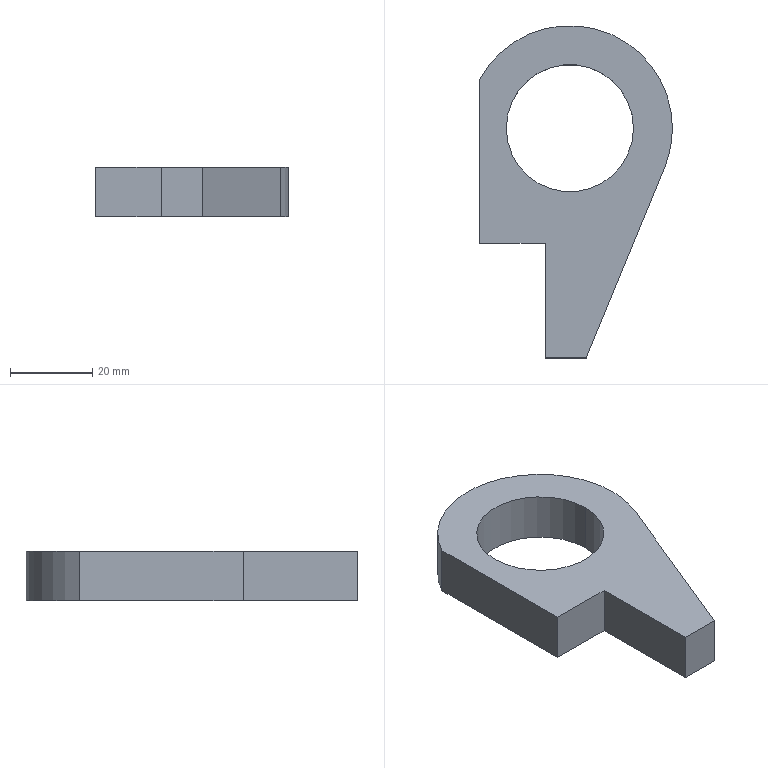Part | SolidWorks | features FlatPattern 1, SMBaseFlange 1, SheetMetal 1 | 1 solid | 11 faces | box 47 x 81 x 12 mm | volume 22191 mm3 | plane 7 | cylinder 4 | commonest cylinder face diameters 31 x2 50 x2
STEP:
#1=CARTESIAN_POINT('',(-15.5,0.,-12.));
#2=VERTEX_POINT('',#1);
#3=CARTESIAN_POINT('',(15.5,0.,-12.));
#4=VERTEX_POINT('',#3);
#5=CARTESIAN_POINT('',(0.,0.,-12.));
#6=DIRECTION('',(0.,0.,1.));
#7=DIRECTION('',(1.,0.,0.));
#8=AXIS2_PLACEMENT_3D('',#5,#6,#7);
#9=CIRCLE('',#8,15.5);
#10=EDGE_CURVE('',#2,#4,#9,.T.);
#11=ORIENTED_EDGE('',*,*,#10,.F.);
#12=CARTESIAN_POINT('',(-15.5,0.,0.));
#13=VERTEX_POINT('',#12);
#14=CARTESIAN_POINT('',(-15.5,0.,-12.));
#15=DIRECTION('',(0.,0.,1.));
#16=VECTOR('',#15,1000.);
#17=LINE('',#14,#16);
#18=EDGE_CURVE('',#2,#13,#17,.T.);
#19=ORIENTED_EDGE('',*,*,#18,.T.);
#20=CARTESIAN_POINT('',(15.5,0.,0.));
#21=VERTEX_POINT('',#20);
#22=CARTESIAN_POINT('',(0.,0.,0.));
#23=DIRECTION('',(0.,0.,1.));
#24=DIRECTION('',(1.,0.,0.));
#25=AXIS2_PLACEMENT_3D('',#22,#23,#24);
#26=CIRCLE('',#25,15.5);
#27=EDGE_CURVE('',#13,#21,#26,.T.);
#28=ORIENTED_EDGE('',*,*,#27,.T.);
#29=CARTESIAN_POINT('',(15.5,0.,-12.));
#30=DIRECTION('',(0.,0.,1.));
#31=VECTOR('',#30,1000.);
#32=LINE('',#29,#31);
#33=EDGE_CURVE('',#4,#21,#32,.T.);
#34=ORIENTED_EDGE('',*,*,#33,.F.);
#35=EDGE_LOOP('',(#11,#19,#28,#34));
#36=FACE_OUTER_BOUND('',#35,.T.);
#37=CARTESIAN_POINT('',(0.,0.,-12.));
#38=DIRECTION('',(0.,0.,1.));
#39=DIRECTION('',(1.,0.,0.));
#40=AXIS2_PLACEMENT_3D('',#37,#38,#39);
#41=CYLINDRICAL_SURFACE('',#40,15.5);
#42=ADVANCED_FACE('',(#36),#41,.F.);
#43=CARTESIAN_POINT('',(23.121,-9.509,-12.));
#44=VERTEX_POINT('',#43);
#45=CARTESIAN_POINT('',(25.,0.,-12.));
#46=VERTEX_POINT('',#45);
#47=CARTESIAN_POINT('',(0.,0.,-12.));
#48=DIRECTION('',(0.,0.,1.));
#49=DIRECTION('',(1.,0.,0.));
#50=AXIS2_PLACEMENT_3D('',#47,#48,#49);
#51=CIRCLE('',#50,25.);
#52=EDGE_CURVE('',#44,#46,#51,.T.);
#53=ORIENTED_EDGE('',*,*,#52,.T.);
#54=CARTESIAN_POINT('',(25.,0.,0.));
#55=VERTEX_POINT('',#54);
#56=CARTESIAN_POINT('',(25.,0.,-12.));
#57=DIRECTION('',(0.,0.,1.));
#58=VECTOR('',#57,1000.);
#59=LINE('',#56,#58);
#60=EDGE_CURVE('',#46,#55,#59,.T.);
#61=ORIENTED_EDGE('',*,*,#60,.T.);
#62=CARTESIAN_POINT('',(23.121,-9.509,0.));
#63=VERTEX_POINT('',#62);
#64=CARTESIAN_POINT('',(0.,0.,0.));
#65=DIRECTION('',(0.,0.,1.));
#66=DIRECTION('',(1.,0.,0.));
#67=AXIS2_PLACEMENT_3D('',#64,#65,#66);
#68=CIRCLE('',#67,25.);
#69=EDGE_CURVE('',#63,#55,#68,.T.);
#70=ORIENTED_EDGE('',*,*,#69,.F.);
#71=CARTESIAN_POINT('',(23.121,-9.509,-12.));
#72=DIRECTION('',(0.,0.,1.));
#73=VECTOR('',#72,1000.);
#74=LINE('',#71,#73);
#75=EDGE_CURVE('',#44,#63,#74,.T.);
#76=ORIENTED_EDGE('',*,*,#75,.F.);
#77=EDGE_LOOP('',(#53,#61,#70,#76));
#78=FACE_OUTER_BOUND('',#77,.T.);
#79=CARTESIAN_POINT('',(0.,0.,-12.));
#80=DIRECTION('',(0.,0.,1.));
#81=DIRECTION('',(1.,0.,0.));
#82=AXIS2_PLACEMENT_3D('',#79,#80,#81);
#83=CYLINDRICAL_SURFACE('',#82,25.);
#84=ADVANCED_FACE('',(#78),#83,.T.);
#85=ORIENTED_EDGE('',*,*,#60,.F.);
#86=CARTESIAN_POINT('',(-22.,11.874,-12.));
#87=VERTEX_POINT('',#86);
#88=CARTESIAN_POINT('',(0.,0.,-12.));
#89=DIRECTION('',(0.,0.,1.));
#90=DIRECTION('',(1.,0.,0.));
#91=AXIS2_PLACEMENT_3D('',#88,#89,#90);
#92=CIRCLE('',#91,25.);
#93=EDGE_CURVE('',#46,#87,#92,.T.);
#94=ORIENTED_EDGE('',*,*,#93,.T.);
#95=CARTESIAN_POINT('',(-22.,11.874,0.));
#96=VERTEX_POINT('',#95);
#97=CARTESIAN_POINT('',(-22.,11.874,-12.));
#98=DIRECTION('',(0.,0.,1.));
#99=VECTOR('',#98,1000.);
#100=LINE('',#97,#99);
#101=EDGE_CURVE('',#87,#96,#100,.T.);
#102=ORIENTED_EDGE('',*,*,#101,.T.);
#103=CARTESIAN_POINT('',(0.,0.,0.));
#104=DIRECTION('',(0.,0.,1.));
#105=DIRECTION('',(1.,0.,0.));
#106=AXIS2_PLACEMENT_3D('',#103,#104,#105);
#107=CIRCLE('',#106,25.);
#108=EDGE_CURVE('',#55,#96,#107,.T.);
#109=ORIENTED_EDGE('',*,*,#108,.F.);
#110=EDGE_LOOP('',(#85,#94,#102,#109));
#111=FACE_OUTER_BOUND('',#110,.T.);
#112=CARTESIAN_POINT('',(0.,0.,-12.));
#113=DIRECTION('',(0.,0.,1.));
#114=DIRECTION('',(1.,0.,0.));
#115=AXIS2_PLACEMENT_3D('',#112,#113,#114);
#116=CYLINDRICAL_SURFACE('',#115,25.);
#117=ADVANCED_FACE('',(#111),#116,.T.);
#118=CARTESIAN_POINT('',(4.,-56.,0.));
#119=VERTEX_POINT('',#118);
#120=CARTESIAN_POINT('',(4.,-56.,0.));
#121=DIRECTION('',(0.3804,0.9248,0.));
#122=VECTOR('',#121,1000.);
#123=LINE('',#120,#122);
#124=EDGE_CURVE('',#119,#63,#123,.T.);
#125=ORIENTED_EDGE('',*,*,#124,.F.);
#126=CARTESIAN_POINT('',(4.,-56.,-12.));
#127=VERTEX_POINT('',#126);
#128=CARTESIAN_POINT('',(4.,-56.,-12.));
#129=DIRECTION('',(0.,0.,1.));
#130=VECTOR('',#129,1000.);
#131=LINE('',#128,#130);
#132=EDGE_CURVE('',#127,#119,#131,.T.);
#133=ORIENTED_EDGE('',*,*,#132,.F.);
#134=CARTESIAN_POINT('',(4.,-56.,-12.));
#135=DIRECTION('',(0.3804,0.9248,0.));
#136=VECTOR('',#135,1000.);
#137=LINE('',#134,#136);
#138=EDGE_CURVE('',#127,#44,#137,.T.);
#139=ORIENTED_EDGE('',*,*,#138,.T.);
#140=ORIENTED_EDGE('',*,*,#75,.T.);
#141=EDGE_LOOP('',(#125,#133,#139,#140));
#142=FACE_OUTER_BOUND('',#141,.T.);
#143=CARTESIAN_POINT('',(4.,-56.,-12.));
#144=DIRECTION('',(0.9248,-0.3804,0.));
#145=DIRECTION('',(0.3804,0.9248,0.));
#146=AXIS2_PLACEMENT_3D('',#143,#144,#145);
#147=PLANE('',#146);
#148=ADVANCED_FACE('',(#142),#147,.T.);
#149=CARTESIAN_POINT('',(-6.,-56.,0.));
#150=VERTEX_POINT('',#149);
#151=CARTESIAN_POINT('',(-6.,-56.,0.));
#152=DIRECTION('',(1.,0.,0.));
#153=VECTOR('',#152,1000.);
#154=LINE('',#151,#153);
#155=EDGE_CURVE('',#150,#119,#154,.T.);
#156=ORIENTED_EDGE('',*,*,#155,.F.);
#157=CARTESIAN_POINT('',(-6.,-56.,-12.));
#158=VERTEX_POINT('',#157);
#159=CARTESIAN_POINT('',(-6.,-56.,-12.));
#160=DIRECTION('',(0.,0.,1.));
#161=VECTOR('',#160,1000.);
#162=LINE('',#159,#161);
#163=EDGE_CURVE('',#158,#150,#162,.T.);
#164=ORIENTED_EDGE('',*,*,#163,.F.);
#165=CARTESIAN_POINT('',(-6.,-56.,-12.));
#166=DIRECTION('',(1.,0.,0.));
#167=VECTOR('',#166,1000.);
#168=LINE('',#165,#167);
#169=EDGE_CURVE('',#158,#127,#168,.T.);
#170=ORIENTED_EDGE('',*,*,#169,.T.);
#171=ORIENTED_EDGE('',*,*,#132,.T.);
#172=EDGE_LOOP('',(#156,#164,#170,#171));
#173=FACE_OUTER_BOUND('',#172,.T.);
#174=CARTESIAN_POINT('',(-6.,-56.,-12.));
#175=DIRECTION('',(0.,-1.,0.));
#176=DIRECTION('',(0.,0.,-1.));
#177=AXIS2_PLACEMENT_3D('',#174,#175,#176);
#178=PLANE('',#177);
#179=ADVANCED_FACE('',(#173),#178,.T.);
#180=CARTESIAN_POINT('',(-6.,-28.,0.));
#181=VERTEX_POINT('',#180);
#182=CARTESIAN_POINT('',(-6.,-28.,0.));
#183=DIRECTION('',(0.,-1.,0.));
#184=VECTOR('',#183,1000.);
#185=LINE('',#182,#184);
#186=EDGE_CURVE('',#181,#150,#185,.T.);
#187=ORIENTED_EDGE('',*,*,#186,.F.);
#188=CARTESIAN_POINT('',(-6.,-28.,-12.));
#189=VERTEX_POINT('',#188);
#190=CARTESIAN_POINT('',(-6.,-28.,-12.));
#191=DIRECTION('',(0.,0.,1.));
#192=VECTOR('',#191,1000.);
#193=LINE('',#190,#192);
#194=EDGE_CURVE('',#189,#181,#193,.T.);
#195=ORIENTED_EDGE('',*,*,#194,.F.);
#196=CARTESIAN_POINT('',(-6.,-28.,-12.));
#197=DIRECTION('',(0.,-1.,0.));
#198=VECTOR('',#197,1000.);
#199=LINE('',#196,#198);
#200=EDGE_CURVE('',#189,#158,#199,.T.);
#201=ORIENTED_EDGE('',*,*,#200,.T.);
#202=ORIENTED_EDGE('',*,*,#163,.T.);
#203=EDGE_LOOP('',(#187,#195,#201,#202));
#204=FACE_OUTER_BOUND('',#203,.T.);
#205=CARTESIAN_POINT('',(-6.,-28.,-12.));
#206=DIRECTION('',(-1.,0.,0.));
#207=DIRECTION('',(0.,-1.,0.));
#208=AXIS2_PLACEMENT_3D('',#205,#206,#207);
#209=PLANE('',#208);
#210=ADVANCED_FACE('',(#204),#209,.T.);
#211=CARTESIAN_POINT('',(-22.,-28.,0.));
#212=VERTEX_POINT('',#211);
#213=CARTESIAN_POINT('',(-22.,-28.,0.));
#214=DIRECTION('',(1.,0.,0.));
#215=VECTOR('',#214,1000.);
#216=LINE('',#213,#215);
#217=EDGE_CURVE('',#212,#181,#216,.T.);
#218=ORIENTED_EDGE('',*,*,#217,.F.);
#219=CARTESIAN_POINT('',(-22.,-28.,-12.));
#220=VERTEX_POINT('',#219);
#221=CARTESIAN_POINT('',(-22.,-28.,-12.));
#222=DIRECTION('',(0.,0.,1.));
#223=VECTOR('',#222,1000.);
#224=LINE('',#221,#223);
#225=EDGE_CURVE('',#220,#212,#224,.T.);
#226=ORIENTED_EDGE('',*,*,#225,.F.);
#227=CARTESIAN_POINT('',(-22.,-28.,-12.));
#228=DIRECTION('',(1.,0.,0.));
#229=VECTOR('',#228,1000.);
#230=LINE('',#227,#229);
#231=EDGE_CURVE('',#220,#189,#230,.T.);
#232=ORIENTED_EDGE('',*,*,#231,.T.);
#233=ORIENTED_EDGE('',*,*,#194,.T.);
#234=EDGE_LOOP('',(#218,#226,#232,#233));
#235=FACE_OUTER_BOUND('',#234,.T.);
#236=CARTESIAN_POINT('',(-22.,-28.,-12.));
#237=DIRECTION('',(0.,-1.,0.));
#238=DIRECTION('',(0.,0.,-1.));
#239=AXIS2_PLACEMENT_3D('',#236,#237,#238);
#240=PLANE('',#239);
#241=ADVANCED_FACE('',(#235),#240,.T.);
#242=CARTESIAN_POINT('',(-22.,-28.,0.));
#243=DIRECTION('',(0.,-1.,0.));
#244=VECTOR('',#243,1000.);
#245=LINE('',#242,#244);
#246=EDGE_CURVE('',#96,#212,#245,.T.);
#247=ORIENTED_EDGE('',*,*,#246,.F.);
#248=ORIENTED_EDGE('',*,*,#101,.F.);
#249=CARTESIAN_POINT('',(-22.,-28.,-12.));
#250=DIRECTION('',(0.,-1.,0.));
#251=VECTOR('',#250,1000.);
#252=LINE('',#249,#251);
#253=EDGE_CURVE('',#87,#220,#252,.T.);
#254=ORIENTED_EDGE('',*,*,#253,.T.);
#255=ORIENTED_EDGE('',*,*,#225,.T.);
#256=EDGE_LOOP('',(#247,#248,#254,#255));
#257=FACE_OUTER_BOUND('',#256,.T.);
#258=CARTESIAN_POINT('',(-22.,-28.,-12.));
#259=DIRECTION('',(-1.,0.,0.));
#260=DIRECTION('',(0.,0.,1.));
#261=AXIS2_PLACEMENT_3D('',#258,#259,#260);
#262=PLANE('',#261);
#263=ADVANCED_FACE('',(#257),#262,.T.);
#264=CARTESIAN_POINT('',(0.,0.,-12.));
#265=DIRECTION('',(0.,0.,1.));
#266=DIRECTION('',(1.,0.,0.));
#267=AXIS2_PLACEMENT_3D('',#264,#265,#266);
#268=CIRCLE('',#267,15.5);
#269=EDGE_CURVE('',#4,#2,#268,.T.);
#270=ORIENTED_EDGE('',*,*,#269,.T.);
#271=ORIENTED_EDGE('',*,*,#10,.T.);
#272=EDGE_LOOP('',(#270,#271));
#273=FACE_BOUND('',#272,.T.);
#274=ORIENTED_EDGE('',*,*,#52,.F.);
#275=ORIENTED_EDGE('',*,*,#138,.F.);
#276=ORIENTED_EDGE('',*,*,#169,.F.);
#277=ORIENTED_EDGE('',*,*,#200,.F.);
#278=ORIENTED_EDGE('',*,*,#231,.F.);
#279=ORIENTED_EDGE('',*,*,#253,.F.);
#280=ORIENTED_EDGE('',*,*,#93,.F.);
#281=EDGE_LOOP('',(#274,#275,#276,#277,#278,#279,#280));
#282=FACE_OUTER_BOUND('',#281,.T.);
#283=CARTESIAN_POINT('',(0.,0.,-12.));
#284=DIRECTION('',(0.,0.,1.));
#285=DIRECTION('',(1.,0.,0.));
#286=AXIS2_PLACEMENT_3D('',#283,#284,#285);
#287=PLANE('',#286);
#288=ADVANCED_FACE('',(#273,#282),#287,.F.);
#289=CARTESIAN_POINT('',(0.,0.,0.));
#290=DIRECTION('',(0.,0.,1.));
#291=DIRECTION('',(1.,0.,0.));
#292=AXIS2_PLACEMENT_3D('',#289,#290,#291);
#293=CIRCLE('',#292,15.5);
#294=EDGE_CURVE('',#21,#13,#293,.T.);
#295=ORIENTED_EDGE('',*,*,#294,.F.);
#296=ORIENTED_EDGE('',*,*,#27,.F.);
#297=EDGE_LOOP('',(#295,#296));
#298=FACE_BOUND('',#297,.T.);
#299=ORIENTED_EDGE('',*,*,#69,.T.);
#300=ORIENTED_EDGE('',*,*,#108,.T.);
#301=ORIENTED_EDGE('',*,*,#246,.T.);
#302=ORIENTED_EDGE('',*,*,#217,.T.);
#303=ORIENTED_EDGE('',*,*,#186,.T.);
#304=ORIENTED_EDGE('',*,*,#155,.T.);
#305=ORIENTED_EDGE('',*,*,#124,.T.);
#306=EDGE_LOOP('',(#299,#300,#301,#302,#303,#304,#305));
#307=FACE_OUTER_BOUND('',#306,.T.);
#308=CARTESIAN_POINT('',(0.,0.,0.));
#309=DIRECTION('',(0.,0.,1.));
#310=DIRECTION('',(1.,0.,0.));
#311=AXIS2_PLACEMENT_3D('',#308,#309,#310);
#312=PLANE('',#311);
#313=ADVANCED_FACE('',(#298,#307),#312,.T.);
#314=ORIENTED_EDGE('',*,*,#18,.F.);
#315=ORIENTED_EDGE('',*,*,#269,.F.);
#316=ORIENTED_EDGE('',*,*,#33,.T.);
#317=ORIENTED_EDGE('',*,*,#294,.T.);
#318=EDGE_LOOP('',(#314,#315,#316,#317));
#319=FACE_OUTER_BOUND('',#318,.T.);
#320=CARTESIAN_POINT('',(0.,0.,-12.));
#321=DIRECTION('',(0.,0.,1.));
#322=DIRECTION('',(1.,0.,0.));
#323=AXIS2_PLACEMENT_3D('',#320,#321,#322);
#324=CYLINDRICAL_SURFACE('',#323,15.5);
#325=ADVANCED_FACE('',(#319),#324,.F.);
#326=CLOSED_SHELL('',(#42,#84,#117,#148,#179,#210,#241,#263,#288,#313,#325));
#327=MANIFOLD_SOLID_BREP('',#326);
#328=CARTESIAN_POINT('',(0.,0.,0.));
#329=DIRECTION('',(0.,0.,1.));
#330=DIRECTION('',(1.,0.,0.));
#331=AXIS2_PLACEMENT_3D('',#328,#329,#330);
#332=(LENGTH_UNIT()NAMED_UNIT(*)SI_UNIT(.MILLI.,.METRE.));
#333=UNCERTAINTY_MEASURE_WITH_UNIT(LENGTH_MEASURE(0.00001),#332,'','');
#334=(NAMED_UNIT(*)PLANE_ANGLE_UNIT()SI_UNIT($,.RADIAN.));
#335=(NAMED_UNIT(*)SI_UNIT($,.STERADIAN.)SOLID_ANGLE_UNIT());
#336=(GEOMETRIC_REPRESENTATION_CONTEXT(3)GLOBAL_UNCERTAINTY_ASSIGNED_CONTEXT((#333))GLOBAL_UNIT_ASSIGNED_CONTEXT((#332,#334,#335))REPRESENTATION_CONTEXT('',''));
#337=ADVANCED_BREP_SHAPE_REPRESENTATION('',(#327,#331),#336);